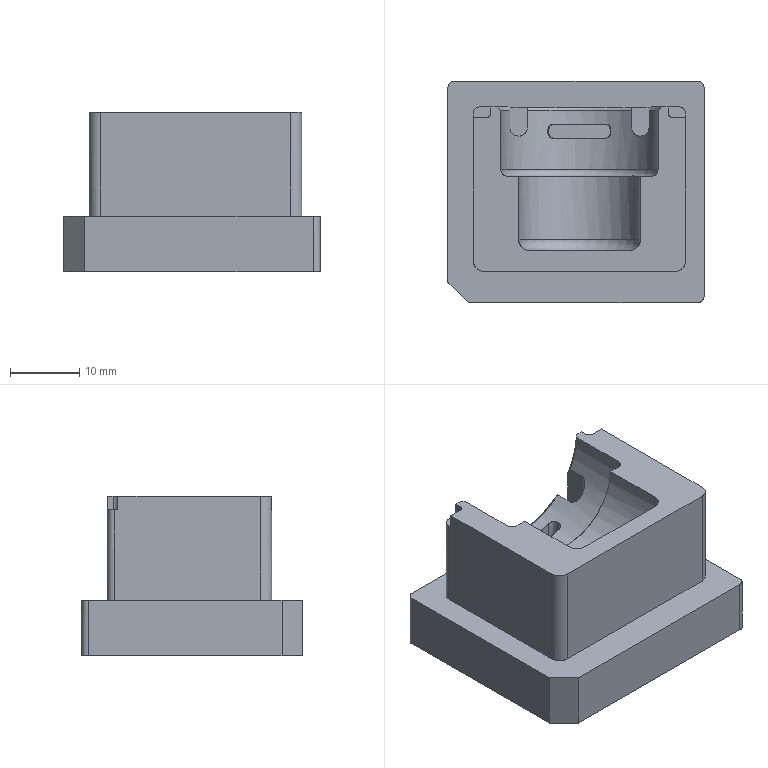NC program | PowerMill | posted with a generic post | part box 37 x 32 x 23 mm
Lines 5912 to 6889 of 253511:
N6009 M6
N6010 S18000 M03
N6011 G00 G90 X0.0 Y0.0
N6012 G43 Z9.8 H15
N6013
N6014 G05 P10000 R4
N6015 X1.851 Y-13.9296
N6016 Z0.8426
N6017 G01 Z-0.3574 F3000.0
N6018 X1.8596 Y-13.9124 F5000.0
N6019 G03 X1.7821 Y-13.6799 I-0.155 J0.0775
N6020 G01 X0.4221 Y-12.9999
N6021 X-13.0861
N6022 X-13.5083 Y-12.9833
N6023 X-13.9304 Y-12.9241
N6024 X-14.3525 Y-12.8
N6025 X-14.7747 Y-12.6037
N6026 X-15.1968 Y-12.3085
N6027 X-15.6189 Y-11.8974
N6028 X-15.9721 Y-11.3976
N6029 X-16.1651 Y-10.9755
N6030 X-16.2874 Y-10.5533
N6031 X-16.3436 Y-10.1312
N6032 X-16.3585 Y-9.7091
N6033 Y10.5533
N6034 X-16.3332 Y10.9755
N6035 X-16.1868 Y11.3976
N6036 X-16.0411 Y11.6235
N6037 X-15.8575 Y11.8197
N6038 X-15.6189 Y11.9937
N6039 X-15.1968 Y12.1621
N6040 X-14.7747 Y12.2007
N6041 X-13.9496
N6042 X-13.8965 Y12.2105
N6043 X-13.8503 Y12.2384
N6044 X-13.8336 Y12.2595
N6045 X-13.8169 Y12.2808
N6046 X-13.8007 Y12.3323
N6047 X-13.7597 Y12.664
N6048 X-13.5651 Y13.0861
N6049 X-13.5083 Y13.1658
N6050 X-13.1402 Y13.5083
N6051 X-12.664 Y13.7137
N6052 X-12.2419 Y13.7545
N6053 X-11.3976
N6054 X-10.9755 Y13.7073
N6055 X-10.5533 Y13.5265
N6056 X-10.1312 Y13.1593
N6057 X-9.7091 Y12.7315
N6058 X-9.4273 Y12.2419
N6059 X-9.3466 Y11.8197
N6060 X-9.3448 Y3.8549
N6061 G03 X-9.1949 Y3.7049 I0.15 J0.0
N6062 G01 X-8.4427 Y3.7045
N6063 X-8.0205 Y3.6777
N6064 X-7.5984 Y3.5401
N6065 X-7.3433 Y3.3771
N6066 X-7.1763 Y3.2216
N6067 X-6.98 Y2.9549
N6068 X-6.8151 Y2.5328
N6069 X-6.7788 Y2.1107
N6070 X-6.7766 Y-6.8379
N6071 G03 X-6.6267 Y-6.9878 I0.15 J0.0001
N6072 G01 X7.5984 Y-7.0024
N6073 X7.6758 Y-6.9844
N6074 X7.7408 Y-6.9386
N6075 X7.7658 Y-6.8942
N6076 X7.7745 Y-6.8439
N6077 X7.7746 Y2.1107
N6078 X7.8108 Y2.5328
N6079 X7.9758 Y2.9549
N6080 X8.3392 Y3.3771
N6081 X8.4427 Y3.4524
N6082 X8.8648 Y3.6473
N6083 X9.2869 Y3.7045
N6084 X10.1905
N6085 G03 X10.3405 Y3.8545 I0.0 J0.15
N6086 G01 X10.3425 Y11.8197
N6087 X10.4231 Y12.2419
N6088 X10.5533 Y12.5205
N6089 X10.65 Y12.664
N6090 X11.3976 Y13.418
N6091 X11.5206 Y13.5083
N6092 X11.8197 Y13.6569
N6093 X12.2419 Y13.7507
N6094 X13.5083 Y13.7416
N6095 X13.9304 Y13.6214
N6096 X14.1361 Y13.5083
N6097 X14.3525 Y13.3355
N6098 X14.561 Y13.0861
N6099 X14.7557 Y12.664
N6100 X14.7965 Y12.3326
N6101 G03 X14.9453 Y12.2009 I0.1489 J0.0183
N6102 G01 X15.4933 Y12.2025
N6103 X16.0411 Y12.189
N6104 X16.4632 Y12.0717
N6105 X16.8533 Y11.8197
N6106 X17.1827 Y11.3976
N6107 X17.3075 Y11.0731
N6108 X17.3544 Y10.5533
N6109 Y-9.7091
N6110 X17.3075 Y-10.4367
N6111 X17.161 Y-10.9755
N6112 X16.8853 Y-11.5381
N6113 X16.4632 Y-12.0749
N6114 X16.0411 Y-12.4308
N6115 X15.6461 Y-12.664
N6116 X15.1968 Y-12.8494
N6117 X14.7747 Y-12.9556
N6118 X14.3525 Y-12.9967
N6119 X13.9304 Y-12.9999
N6120 X0.4221
N6121 X1.851 Y-13.9296 Z-0.5048
N6122 X1.8596 Y-13.9124
N6123 G03 X1.7821 Y-13.6799 I-0.155 J0.0775
N6124 G01 X0.4221 Y-12.9999
N6125 X-13.0861
N6126 X-13.5083 Y-12.9833
N6127 X-13.9304 Y-12.9241
N6128 X-14.3525 Y-12.8
N6129 X-14.7747 Y-12.6037
N6130 X-15.1968 Y-12.3085
N6131 X-15.6189 Y-11.8974
N6132 X-15.9721 Y-11.3976
N6133 X-16.1651 Y-10.9755
N6134 X-16.2874 Y-10.5533
N6135 X-16.3436 Y-10.1312
N6136 X-16.3585 Y-9.7091
N6137 Y10.5533
N6138 X-16.3332 Y10.9755
N6139 X-16.1868 Y11.3976
N6140 X-16.0411 Y11.6235
N6141 X-15.8575 Y11.8197
N6142 X-15.6189 Y11.9937
N6143 X-15.1968 Y12.1621
N6144 X-14.7747 Y12.2008
N6145 X-13.9496
N6146 G03 X-13.8007 Y12.3323 I0.0 J0.15
N6147 G01 X-13.7597 Y12.664
N6148 X-13.5651 Y13.0861
N6149 X-13.5083 Y13.1658
N6150 X-13.1402 Y13.5083
N6151 X-12.664 Y13.7137
N6152 X-12.2419 Y13.7545
N6153 X-11.3976
N6154 X-10.9755 Y13.7097
N6155 X-10.5533 Y13.5324
N6156 X-10.1312 Y13.1691
N6157 X-9.7118 Y12.7342
N6158 X-9.7091 Y12.7315
N6159 X-9.709 Y12.7313
N6160 X-9.6441 Y12.664
N6161 X-9.4172 Y12.2419
N6162 X-9.3365 Y11.8197
N6163 X-9.3345 Y3.8547
N6164 G03 X-9.191 Y3.7049 I0.15 J0.0
N6165 G01 X-8.6479 Y3.7046
N6166 X-8.4427 Y3.7045
N6167 X-8.0205 Y3.6812
N6168 X-7.5984 Y3.5477
N6169 X-7.3307 Y3.3771
N6170 X-7.1763 Y3.2349
N6171 X-6.9673 Y2.9549
N6172 X-6.8025 Y2.5328
N6173 X-6.7661 Y2.1107
N6174 X-6.7657 Y-6.8448
N6175 X-6.7625 Y-6.8644
N6176 X-6.7197 Y-6.9464
N6177 X-6.6365 Y-6.9866
N6178 X-6.6267 Y-6.9879
N6179 X5.9184 Y-7.0008
N6180 X7.5912 Y-7.0009
N6181 X7.6062 Y-7.0001
N6182 X7.621 Y-6.9978
N6183 X7.6432 Y-6.9933
N6184 X7.7205 Y-6.9501
N6185 X7.759 Y-6.8703
N6186 X7.762 Y-6.8489
N6187 Y2.1107
N6188 X7.7979 Y2.5328
N6189 X7.9632 Y2.9549
N6190 X8.0205 Y3.0455
N6191 X8.3265 Y3.3771
N6192 X8.4427 Y3.4605
N6193 X8.8648 Y3.6507
N6194 X9.2869 Y3.7045
N6195 X10.1802
N6196 G03 X10.3302 Y3.8545 I0.0 J0.15
N6197 G01 X10.3324 Y11.8197
N6198 X10.4128 Y12.2419
N6199 X10.5533 Y12.5366
N6200 X10.6399 Y12.664
N6201 X11.3976 Y13.4257
N6202 X11.5107 Y13.5083
N6203 X11.8197 Y13.6635
N6204 X12.2419 Y13.7514
N6205 X13.5083 Y13.7416
N6206 X13.9304 Y13.6214
N6207 X14.1361 Y13.5083
N6208 X14.3525 Y13.3356
N6209 X14.561 Y13.0861
N6210 X14.7557 Y12.664
N6211 X14.7965 Y12.3326
N6212 G03 X14.9453 Y12.201 I0.1489 J0.0183
N6213 G01 X15.4933 Y12.2025
N6214 X16.0411 Y12.189
N6215 X16.4632 Y12.0717
N6216 X16.8533 Y11.8197
N6217 X17.1827 Y11.3976
N6218 X17.3075 Y11.0731
N6219 X17.3544 Y10.5533
N6220 Y-9.7091
N6221 X17.3075 Y-10.4367
N6222 X17.161 Y-10.9755
N6223 X16.8853 Y-11.5381
N6224 X16.4632 Y-12.0749
N6225 X16.0411 Y-12.4308
N6226 X15.6461 Y-12.664
N6227 X15.1968 Y-12.8494
N6228 X14.7747 Y-12.9556
N6229 X14.3525 Y-12.9967
N6230 X13.9304 Y-12.9999
N6231 X0.4221
N6232 X1.851 Y-13.9296 Z-0.6521
N6233 X1.8596 Y-13.9124
N6234 G03 X1.7821 Y-13.6799 I-0.155 J0.0775
N6235 G01 X0.4221 Y-12.9999
N6236 X-13.0861
N6237 X-13.5083 Y-12.9833
N6238 X-13.9304 Y-12.9241
N6239 X-14.3525 Y-12.8
N6240 X-14.7747 Y-12.6037
N6241 X-15.1968 Y-12.3085
N6242 X-15.6189 Y-11.8974
N6243 X-15.9721 Y-11.3976
N6244 X-16.1651 Y-10.9755
N6245 X-16.2874 Y-10.5533
N6246 X-16.3436 Y-10.1312
N6247 X-16.3585 Y-9.7091
N6248 Y10.5533
N6249 X-16.3332 Y10.9755
N6250 X-16.1868 Y11.3976
N6251 X-16.0411 Y11.6235
N6252 X-15.8575 Y11.8197
N6253 X-15.6189 Y11.9937
N6254 X-15.1968 Y12.1621
N6255 X-14.7747 Y12.2008
N6256 X-13.9496
N6257 G03 X-13.8007 Y12.3324 I0.0 J0.15
N6258 G01 X-13.7598 Y12.664
N6259 X-13.5651 Y13.0861
N6260 X-13.5083 Y13.1658
N6261 X-13.1402 Y13.5083
N6262 X-12.664 Y13.7137
N6263 X-12.2419 Y13.7545
N6264 X-11.3976
N6265 X-10.9755 Y13.712
N6266 X-10.5533 Y13.5384
N6267 X-10.1312 Y13.1788
N6268 X-9.634 Y12.664
N6269 X-9.4071 Y12.2419
N6270 X-9.3264 Y11.8197
N6271 X-9.3242 Y3.8524
N6272 X-9.312 Y3.7924
N6273 X-9.2746 Y3.7438
N6274 X-9.2285 Y3.7149
N6275 X-9.175 Y3.7048
N6276 X-8.6479 Y3.7045
N6277 X-8.3341 Y3.6997
N6278 X-8.0205 Y3.6847
N6279 X-7.5984 Y3.5539
N6280 X-7.318 Y3.3771
N6281 X-7.1763 Y3.2483
N6282 X-6.9547 Y2.9549
N6283 X-6.7898 Y2.5328
N6284 X-6.7541 Y2.248
N6285 X-6.7532 Y-6.8394
N6286 G03 X-6.6239 Y-6.9879 I0.15 J0.0
N6287 G01 X4.5985 Y-6.9995
N6288 X7.5871 Y-6.9993
N6289 X7.6098 Y-6.9975
N6290 X7.6319 Y-6.9923
N6291 G03 X7.7487 Y-6.848 I-0.0282 J0.1422
N6292 G01 X7.7494 Y2.1107
N6293 X7.785 Y2.5328
N6294 X7.9506 Y2.9549
N6295 X8.0205 Y3.0642
N6296 X8.3139 Y3.3771
N6297 X8.4427 Y3.4685
N6298 X8.8648 Y3.6541
N6299 X9.2869 Y3.7045
N6300 X10.1701
N6301 G03 X10.3201 Y3.8545 I0.0 J0.15
N6302 G01 X10.3223 Y11.8197
N6303 X10.4026 Y12.2419
N6304 X10.4816 Y12.3874
N6305 X10.5534 Y12.5366
N6306 X10.5949 Y12.5983
N6307 X10.6299 Y12.664
N6308 X10.9755 Y13.027
N6309 X11.2635 Y13.2908
N6310 X11.3976 Y13.4256
N6311 X11.4623 Y13.4729
N6312 X11.501 Y13.5083
N6313 X11.8197 Y13.6669
N6314 X12.2419 Y13.752
N6315 X13.5083 Y13.7416
N6316 X13.9304 Y13.6214
N6317 X14.1361 Y13.5083
N6318 X14.3525 Y13.3356
N6319 X14.561 Y13.0861
N6320 X14.7557 Y12.664
N6321 X14.7965 Y12.3326
N6322 G03 X14.9453 Y12.201 I0.1489 J0.0184
N6323 G01 X15.4933 Y12.2025
N6324 X16.0411 Y12.189
N6325 X16.4632 Y12.0717
N6326 X16.8533 Y11.8197
N6327 X17.1827 Y11.3976
N6328 X17.3075 Y11.0731
N6329 X17.3544 Y10.5533
N6330 Y-9.7091
N6331 X17.3075 Y-10.4367
N6332 X17.161 Y-10.9755
N6333 X16.8853 Y-11.5381
N6334 X16.4632 Y-12.0749
N6335 X16.0411 Y-12.4308
N6336 X15.6461 Y-12.664
N6337 X15.1968 Y-12.8494
N6338 X14.7747 Y-12.9556
N6339 X14.3525 Y-12.9967
N6340 X13.9304 Y-12.9999
N6341 X0.4221
N6342 X1.851 Y-13.9296 Z-0.7995
N6343 X1.8596 Y-13.9124
N6344 G03 X1.7821 Y-13.6799 I-0.155 J0.0775
N6345 G01 X0.4221 Y-12.9999
N6346 X-13.0861
N6347 X-13.5083 Y-12.9833
N6348 X-13.9304 Y-12.9241
N6349 X-14.3525 Y-12.8
N6350 X-14.7747 Y-12.6037
N6351 X-15.1968 Y-12.3085
N6352 X-15.6189 Y-11.8974
N6353 X-15.9721 Y-11.3976
N6354 X-16.1651 Y-10.9755
N6355 X-16.2874 Y-10.5533
N6356 X-16.3436 Y-10.1312
N6357 X-16.3585 Y-9.7091
N6358 Y10.5533
N6359 X-16.3332 Y10.9755
N6360 X-16.1869 Y11.3976
N6361 X-16.0411 Y11.6236
N6362 X-15.8575 Y11.8197
N6363 X-15.6189 Y11.9937
N6364 X-15.1968 Y12.1621
N6365 X-14.7747 Y12.2008
N6366 X-13.9496
N6367 G03 X-13.8007 Y12.3324 I0.0 J0.15
N6368 G01 X-13.7598 Y12.664
N6369 X-13.5651 Y13.0861
N6370 X-13.5083 Y13.1658
N6371 X-13.1403 Y13.5083
N6372 X-12.664 Y13.7137
N6373 X-12.2419 Y13.7545
N6374 X-11.3976
N6375 X-10.9755 Y13.7144
N6376 X-10.5533 Y13.5443
N6377 X-10.1312 Y13.1886
N6378 X-9.6239 Y12.664
N6379 X-9.3971 Y12.2419
N6380 X-9.3164 Y11.8197
N6381 X-9.3139 Y3.853
N6382 X-9.2863 Y3.766
N6383 X-9.2117 Y3.7134
N6384 X-9.1866 Y3.7048
N6385 X-8.6034
N6386 X-8.0205 Y3.6882
N6387 X-7.5984 Y3.5602
N6388 X-7.3054 Y3.3771
N6389 X-7.1763 Y3.2617
N6390 X-6.942 Y2.9549
N6391 X-6.7772 Y2.5328
N6392 X-6.7408 Y2.1107
N6393 X-6.741 Y-6.8382
N6394 G03 X-6.5986 Y-6.988 I0.15 J0.0
N6395 G01 X3.5218 Y-6.9984
N6396 X7.5848 Y-6.9977
N6397 G03 X7.7348 Y-6.8478 I0.0 J0.15
N6398 G01 X7.7367 Y2.1107
N6399 X7.7721 Y2.5328
N6400 X7.9379 Y2.9549
N6401 X8.0205 Y3.0825
N6402 X8.3013 Y3.3771
N6403 X8.4427 Y3.4766
N6404 X8.8648 Y3.6575
N6405 X9.2869 Y3.7045
N6406 X10.1597
N6407 G03 X10.3097 Y3.8545 I0.0 J0.15
N6408 G01 X10.3122 Y11.8197
N6409 X10.3924 Y12.2419
N6410 X10.6198 Y12.664
N6411 X10.8271 Y12.8711
N6412 X10.9431 Y12.9951
N6413 X11.0673 Y13.111
N6414 X11.3976 Y13.441
N6415 X11.4713 Y13.481
N6416 X11.501 Y13.5082
N6417 X11.7434 Y13.6289
N6418 X11.8197 Y13.6703
N6419 X12.2419 Y13.7526
N6420 X13.5083 Y13.7416
N6421 X13.9304 Y13.6214
N6422 X14.1362 Y13.5083
N6423 X14.3525 Y13.3356
N6424 X14.561 Y13.0861
N6425 X14.7557 Y12.664
N6426 X14.7965 Y12.3326
N6427 G03 X14.9453 Y12.201 I0.1489 J0.0184
N6428 G01 X15.4933 Y12.2025
N6429 X16.0411 Y12.189
N6430 X16.4632 Y12.0717
N6431 X16.8533 Y11.8197
N6432 X17.1827 Y11.3976
N6433 X17.3075 Y11.0731
N6434 X17.3544 Y10.5533
N6435 Y-9.7091
N6436 X17.3075 Y-10.4367
N6437 X17.161 Y-10.9755
N6438 X16.8853 Y-11.5381
N6439 X16.4632 Y-12.0749
N6440 X16.0411 Y-12.4308
N6441 X15.6461 Y-12.664
N6442 X15.1968 Y-12.8494
N6443 X14.7747 Y-12.9556
N6444 X14.3525 Y-12.9967
N6445 X13.9304 Y-12.9999
N6446 X0.4221
N6447 X1.851 Y-13.9296 Z-0.9469
N6448 X1.8596 Y-13.9124
N6449 G03 X1.7821 Y-13.6799 I-0.155 J0.0775
N6450 G01 X0.4221 Y-12.9999
N6451 X-13.0861
N6452 X-13.5083 Y-12.9833
N6453 X-13.9304 Y-12.9241
N6454 X-14.3525 Y-12.8
N6455 X-14.7747 Y-12.6037
N6456 X-15.1968 Y-12.3085
N6457 X-15.6189 Y-11.8974
N6458 X-15.9721 Y-11.3976
N6459 X-16.1651 Y-10.9755
N6460 X-16.2874 Y-10.5533
N6461 X-16.3436 Y-10.1312
N6462 X-16.3585 Y-9.7091
N6463 Y10.5533
N6464 X-16.3332 Y10.9755
N6465 X-16.1869 Y11.3976
N6466 X-16.0411 Y11.6236
N6467 X-15.8575 Y11.8197
N6468 X-15.6189 Y11.9937
N6469 X-15.1968 Y12.1621
N6470 X-14.7747 Y12.2008
N6471 X-13.9496
N6472 G03 X-13.8007 Y12.3324 I0.0 J0.15
N6473 G01 X-13.7598 Y12.664
N6474 X-13.5651 Y13.0861
N6475 X-13.5083 Y13.1658
N6476 X-13.1403 Y13.5083
N6477 X-12.664 Y13.7137
N6478 X-12.2419 Y13.7545
N6479 X-11.3976
N6480 X-10.9755 Y13.7168
N6481 X-10.5533 Y13.5502
N6482 X-10.1312 Y13.1983
N6483 X-9.6138 Y12.664
N6484 X-9.387 Y12.2419
N6485 X-9.3063 Y11.8197
N6486 X-9.3035 Y3.8533
N6487 G03 X-9.1735 Y3.7047 I0.15 J0.0001
N6488 G01 X-8.5969 Y3.7042
N6489 X-8.0205 Y3.6905
N6490 X-7.5984 Y3.5664
N6491 X-7.2927 Y3.3771
N6492 X-7.1763 Y3.275
N6493 X-6.9294 Y2.9549
N6494 X-6.7646 Y2.5328
N6495 X-6.7282 Y2.1107
N6496 X-6.7284 Y-6.8351
N6497 G03 X-6.5956 Y-6.9841 I0.15 J0.0
N6498 G01 X-6.5608 Y-6.9881
N6499 X3.5218 Y-6.9985
N6500 X6.9075 Y-6.9979
N6501 X7.5757 Y-6.9887
N6502 G03 X7.7237 Y-6.8387 I-0.002 J0.15
N6503 G01 X7.7241 Y2.1107
N6504 X7.7593 Y2.5328
N6505 X7.9253 Y2.9549
N6506 X8.0205 Y3.1001
N6507 X8.2886 Y3.3771
N6508 X8.4427 Y3.4847
N6509 X8.8648 Y3.6614
N6510 X9.2869 Y3.7045
N6511 X10.1496
N6512 G03 X10.2996 Y3.8545 I0.0 J0.15
N6513 G01 X10.3022 Y11.8197
N6514 X10.3821 Y12.2419
N6515 X10.6097 Y12.664
N6516 X11.3976 Y13.4486
N6517 X11.4733 Y13.489
N6518 X11.4877 Y13.4978
N6519 X11.501 Y13.5082
N6520 X11.6241 Y13.5694
N6521 X11.8197 Y13.6737
N6522 X12.2419 Y13.7532
N6523 X13.5083 Y13.7416
N6524 X13.9304 Y13.6215
N6525 X14.1362 Y13.5083
N6526 X14.3525 Y13.3356
N6527 X14.561 Y13.0861
N6528 X14.7557 Y12.664
N6529 X14.7965 Y12.3326
N6530 G03 X14.9453 Y12.201 I0.1489 J0.0184
N6531 G01 X15.4933 Y12.2025
N6532 X16.0411 Y12.1891
N6533 X16.4632 Y12.0717
N6534 X16.8533 Y11.8197
N6535 X17.1827 Y11.3976
N6536 X17.3075 Y11.0731
N6537 X17.3544 Y10.5533
N6538 Y-9.7091
N6539 X17.3075 Y-10.4367
N6540 X17.161 Y-10.9755
N6541 X16.8853 Y-11.5381
N6542 X16.4632 Y-12.075
N6543 X16.0411 Y-12.4308
N6544 X15.6461 Y-12.664
N6545 X15.1968 Y-12.8494
N6546 X14.7747 Y-12.9556
N6547 X14.3525 Y-12.9967
N6548 X13.9304 Y-12.9999
N6549 X0.4221
N6550 X1.851 Y-13.9296 Z-1.0943
N6551 X1.8596 Y-13.9124
N6552 G03 X1.7821 Y-13.6799 I-0.155 J0.0775
N6553 G01 X0.4221 Y-12.9999
N6554 X-13.0861
N6555 X-13.5083 Y-12.9833
N6556 X-13.9304 Y-12.9241
N6557 X-14.3525 Y-12.8
N6558 X-14.7747 Y-12.6037
N6559 X-15.1968 Y-12.3085
N6560 X-15.6189 Y-11.8974
N6561 X-15.9721 Y-11.3976
N6562 X-16.1651 Y-10.9755
N6563 X-16.2874 Y-10.5533
N6564 X-16.3436 Y-10.1312
N6565 X-16.3586 Y-9.7091
N6566 Y10.5533
N6567 X-16.3332 Y10.9755
N6568 X-16.1869 Y11.3976
N6569 X-16.0411 Y11.6236
N6570 X-15.8575 Y11.8197
N6571 X-15.6189 Y11.9937
N6572 X-15.1968 Y12.1621
N6573 X-14.7747 Y12.2008
N6574 X-13.9496
N6575 G03 X-13.8008 Y12.3324 I0.0 J0.15
N6576 G01 X-13.7598 Y12.664
N6577 X-13.5651 Y13.0861
N6578 X-13.5083 Y13.1658
N6579 X-13.1403 Y13.5083
N6580 X-12.664 Y13.7138
N6581 X-12.2419 Y13.7545
N6582 X-11.3976
N6583 X-10.9755 Y13.7191
N6584 X-10.5533 Y13.5571
N6585 X-10.1312 Y13.2081
N6586 X-9.6038 Y12.664
N6587 X-9.3769 Y12.2419
N6588 X-9.2962 Y11.8197
N6589 X-9.2932 Y3.8546
N6590 G03 X-9.1463 Y3.7047 I0.15 J0.0
N6591 G01 X-8.5834 Y3.7037
N6592 X-8.0205 Y3.6927
N6593 X-7.5984 Y3.5727
N6594 X-7.2799 Y3.3771
N6595 X-7.1763 Y3.2884
N6596 X-6.9147 Y2.9549
N6597 X-6.7503 Y2.5328
N6598 X-6.7156 Y2.1107
N6599 Y-6.7541
N6600 X-6.7143 Y-6.8221
N6601 X-6.7014 Y-6.8889
N6602 X-6.6551 Y-6.9505
N6603 X-6.5843 Y-6.9809
N6604 X-6.5352 Y-6.9882
N6605 X3.5218 Y-6.9985
N6606 X6.9075 Y-6.998
N6607 X7.5555 Y-6.9891
N6608 X7.6429 Y-6.9588
N6609 X7.6949 Y-6.8824
N6610 X7.7019 Y-6.8578
N6611 X7.711 Y-6.7541
N6612 X7.7114 Y2.1107
N6613 X7.7464 Y2.5328
N6614 X7.9111 Y2.9549
N6615 X8.0205 Y3.1177
N6616 X8.274 Y3.3771
N6617 X8.4427 Y3.4948
N6618 X8.8648 Y3.6662
N6619 X9.2869 Y3.7045
N6620 X10.1398
N6621 G03 X10.2898 Y3.8545 I0.0 J0.15
N6622 G01 X10.2921 Y11.8197
N6623 X10.3719 Y12.2419
N6624 X10.5996 Y12.664
N6625 X11.3976 Y13.4565
N6626 X11.8197 Y13.6777
N6627 X12.2419 Y13.7535
N6628 X13.5083 Y13.7417
N6629 X13.9304 Y13.6215
N6630 X14.1362 Y13.5083
N6631 X14.3525 Y13.3356
N6632 X14.561 Y13.0861
N6633 X14.7557 Y12.664
N6634 X14.7965 Y12.3326
N6635 G03 X14.9453 Y12.201 I0.1489 J0.0184
N6636 G01 X15.4933 Y12.2025
N6637 X16.0411 Y12.1891
N6638 X16.4632 Y12.0717
N6639 X16.8534 Y11.8197
N6640 X17.1827 Y11.3976
N6641 X17.3075 Y11.0731
N6642 X17.3544 Y10.5533
N6643 Y-9.7091
N6644 X17.3075 Y-10.4367
N6645 X17.161 Y-10.9755
N6646 X16.8853 Y-11.5381
N6647 X16.4632 Y-12.075
N6648 X16.0411 Y-12.4308
N6649 X15.6461 Y-12.664
N6650 X15.1968 Y-12.8494
N6651 X14.7747 Y-12.9556
N6652 X14.3525 Y-12.9967
N6653 X13.9304 Y-12.9999
N6654 X0.4221
N6655 X1.851 Y-13.9296 Z-1.2417
N6656 X1.8596 Y-13.9124
N6657 G03 X1.7821 Y-13.6799 I-0.155 J0.0775
N6658 G01 X0.4221 Y-12.9999
N6659 X-13.0861
N6660 X-13.5083 Y-12.9833
N6661 X-13.9304 Y-12.9241
N6662 X-14.3525 Y-12.8
N6663 X-14.7747 Y-12.6037
N6664 X-15.1968 Y-12.3085
N6665 X-15.6189 Y-11.8974
N6666 X-15.9721 Y-11.3976
N6667 X-16.1651 Y-10.9755
N6668 X-16.2874 Y-10.5533
N6669 X-16.3436 Y-10.1312
N6670 X-16.3586 Y-9.7091
N6671 Y10.5533
N6672 X-16.3332 Y10.9755
N6673 X-16.1869 Y11.3976
N6674 X-16.0411 Y11.6236
N6675 X-15.8575 Y11.8197
N6676 X-15.6189 Y11.9937
N6677 X-15.1968 Y12.1621
N6678 X-14.7747 Y12.2008
N6679 X-13.9496
N6680 G03 X-13.8008 Y12.3324 I0.0 J0.15
N6681 G01 X-13.7598 Y12.664
N6682 X-13.5651 Y13.0861
N6683 X-13.5083 Y13.1658
N6684 X-13.1403 Y13.5083
N6685 X-12.664 Y13.7138
N6686 X-12.2419 Y13.7545
N6687 X-11.3976
N6688 X-10.9755 Y13.7225
N6689 X-10.5533 Y13.5641
N6690 X-10.1312 Y13.2195
N6691 X-9.5931 Y12.664
N6692 X-9.3646 Y12.2419
N6693 X-9.2869 Y11.8361
N6694 X-9.2825 Y11.3976
N6695 X-9.2829 Y3.8535
N6696 G03 X-9.1742 Y3.7118 I0.1433 J-0.0026
N6697 G01 X-9.1519 Y3.7064
N6698 X-9.1289 Y3.7046
N6699 X-8.5747 Y3.7035
N6700 X-8.0205 Y3.695
N6701 X-7.5984 Y3.5822
N6702 X-7.3218 Y3.4027
N6703 X-7.2799 Y3.377
N6704 X-7.2729 Y3.371
N6705 X-7.1763 Y3.3083
N6706 X-6.8929 Y2.9549
N6707 X-6.7541 Y2.6292
N6708 X-6.6947 Y2.1107
N6709 X-6.6981 Y1.6885
N6710 Y-6.7541
N6711 X-6.6922 Y-6.8527
N6712 X-6.6829 Y-6.8834
N6713 X-6.6744 Y-6.9015
N6714 X-6.629 Y-6.9568
N6715 X-6.5629 Y-6.9841
N6716 X-6.5352 Y-6.9882
N6717 X3.5218 Y-6.9986
N6718 X6.9075 Y-6.998
N6719 X7.5347 Y-6.9894
N6720 X7.6218 Y-6.9593
N6721 X7.6739 Y-6.8833
N6722 X7.6801 Y-6.8615
N6723 X7.694 Y-6.7541
N6724 Y1.2664
N6725 X7.6904 Y2.1107
N6726 X7.7242 Y2.5328
N6727 X7.8889 Y2.9549
N6728 X8.0205 Y3.1461
N6729 X8.2529 Y3.3771
N6730 X8.4427 Y3.5069
N6731 X8.8648 Y3.6709
N6732 X9.2869 Y3.7045
N6733 X10.1293
N6734 G03 X10.2793 Y3.8545 I0.0 J0.15
N6735 G01 X10.279 Y11.8197
N6736 X10.3614 Y12.2419
N6737 X10.5862 Y12.664
N6738 X11.3976 Y13.4672
N6739 X11.8197 Y13.6834
N6740 X12.2419 Y13.754
N6741 X13.5083 Y13.7417
N6742 X13.9304 Y13.6215
N6743 X14.1362 Y13.5083
N6744 X14.3525 Y13.3356
N6745 X14.561 Y13.0861
N6746 X14.7558 Y12.664
N6747 X14.7965 Y12.3326
N6748 G03 X14.9453 Y12.201 I0.1489 J0.0184
N6749 G01 X15.4933 Y12.2026
N6750 X16.0411 Y12.1891
N6751 X16.4632 Y12.0717
N6752 X16.8534 Y11.8197
N6753 X17.1828 Y11.3976
N6754 X17.3075 Y11.0731
N6755 X17.3544 Y10.5533
N6756 Y-9.7091
N6757 X17.3075 Y-10.4367
N6758 X17.161 Y-10.9755
N6759 X16.8853 Y-11.5381
N6760 X16.4632 Y-12.075
N6761 X16.0411 Y-12.4308
N6762 X15.6461 Y-12.664
N6763 X15.1968 Y-12.8494
N6764 X14.7747 Y-12.9556
N6765 X14.3525 Y-12.9967
N6766 X13.9304 Y-12.9999
N6767 X0.4221
N6768 X1.851 Y-13.9296 Z-1.3891
N6769 X1.8596 Y-13.9124
N6770 G03 X1.7821 Y-13.6799 I-0.155 J0.0775
N6771 G01 X0.4221 Y-12.9999
N6772 X-13.0861
N6773 X-13.5083 Y-12.9833
N6774 X-13.9304 Y-12.9241
N6775 X-14.3525 Y-12.8
N6776 X-14.7747 Y-12.6037
N6777 X-15.1968 Y-12.3085
N6778 X-15.6189 Y-11.8974
N6779 X-15.9721 Y-11.3976
N6780 X-16.1651 Y-10.9755
N6781 X-16.2874 Y-10.5533
N6782 X-16.3436 Y-10.1312
N6783 X-16.3586 Y-9.7091
N6784 Y10.5533
N6785 X-16.3332 Y10.9755
N6786 X-16.1869 Y11.3976
N6787 X-16.0411 Y11.6236
N6788 X-15.8575 Y11.8197
N6789 X-15.6189 Y11.9937
N6790 X-15.1968 Y12.1622
N6791 X-14.7747 Y12.2008
N6792 X-13.9496
N6793 G03 X-13.8008 Y12.3324 I0.0 J0.15
N6794 G01 X-13.7598 Y12.664
N6795 X-13.5651 Y13.0861
N6796 X-13.5083 Y13.1658
N6797 X-13.1403 Y13.5083
N6798 X-12.664 Y13.7138
N6799 X-12.2419 Y13.7545
N6800 X-11.3976
N6801 X-10.9755 Y13.7259
N6802 X-10.5533 Y13.5745
N6803 X-10.4422 Y13.5083
N6804 X-10.1312 Y13.2384
N6805 X-9.57 Y12.664
N6806 X-9.3432 Y12.2419
N6807 X-9.2869 Y12.0288
N6808 X-9.2625 Y11.8197
N6809 X-9.2624 Y3.854
N6810 G03 X-9.1257 Y3.7045 I0.15 J0.0
N6811 G01 X-8.7396 Y3.7057
N6812 X-8.3534 Y3.6993
N6813 X-8.0205 Y3.6972
N6814 X-7.5984 Y3.5929
N6815 X-7.2328 Y3.3771
N6816 X-6.8689 Y2.9549
N6817 X-6.7541 Y2.704
N6818 X-6.7036 Y2.5328
N6819 X-6.6683 Y2.1107
N6820 Y-6.8412
N6821 X-6.6646 Y-6.8644
N6822 G03 X-6.5195 Y-6.9883 I0.1452 J0.0231
N6823 G01 X3.5218 Y-6.9986
N6824 X6.9075 Y-6.9981
N6825 X7.5145 Y-6.9897
N6826 X7.5876 Y-6.9691
N6827 X7.6406 Y-6.9148
N6828 X7.6575 Y-6.8804
N6829 X7.6618 Y-6.8423
N6830 X7.6641 Y2.1107
N6831 X7.7005 Y2.5328
N6832 X7.865 Y2.9549
N6833 X8.0205 Y3.1755
N6834 X8.2283 Y3.3771
N6835 X8.4427 Y3.5194
N6836 X8.8648 Y3.6757
N6837 X9.2869 Y3.7045
N6838 X10.1067
N6839 G03 X10.2567 Y3.8545 I0.0 J0.15
N6840 G01 X10.2572 Y11.8197
N6841 X10.3378 Y12.2419
N6842 X10.5647 Y12.664
N6843 X10.9718 Y13.0861
N6844 X11.3976 Y13.4809
N6845 X11.8197 Y13.6891
N6846 X12.2419 Y13.7544
N6847 X13.5083 Y13.7417
N6848 X13.9304 Y13.6215
N6849 X14.1362 Y13.5083
N6850 X14.3525 Y13.3356
N6851 X14.561 Y13.0861
N6852 X14.7558 Y12.664
N6853 X14.7965 Y12.3327
N6854 G03 X14.9453 Y12.201 I0.1489 J0.0183
N6855 G01 X15.4933 Y12.2026
N6856 X16.0411 Y12.1891
N6857 X16.4632 Y12.0717
N6858 X16.8534 Y11.8197
N6859 X17.1828 Y11.3976
N6860 X17.3075 Y11.0731
N6861 X17.3544 Y10.5533
N6862 Y-9.7091
N6863 X17.3075 Y-10.4367
N6864 X17.161 Y-10.9755
N6865 X16.8853 Y-11.5381
N6866 X16.4632 Y-12.075
N6867 X16.0411 Y-12.4308
N6868 X15.6461 Y-12.664
N6869 X15.1968 Y-12.8494
N6870 X14.7747 Y-12.9556
N6871 X14.3525 Y-12.9967
N6872 X13.9304 Y-12.9999
N6873 X0.4221
N6874 X1.851 Y-13.9296 Z-1.5365
N6875 X1.8596 Y-13.9124
N6876 G03 X1.7821 Y-13.6799 I-0.155 J0.0775
N6877 G01 X0.4221 Y-12.9999
N6878 X-13.0861
N6879 X-13.5083 Y-12.9833
N6880 X-13.9304 Y-12.9241
N6881 X-14.3525 Y-12.8
N6882 X-14.7747 Y-12.6037
N6883 X-15.1968 Y-12.3085
N6884 X-15.6189 Y-11.8974
N6885 X-15.9721 Y-11.3976
N6886 X-16.1651 Y-10.9755
N6887 X-16.2874 Y-10.5533
N6888 X-16.3436 Y-10.1312
N6889 X-16.3586 Y-9.7091
N6890 Y10.5533
N6891 X-16.3332 Y10.9755
N6892 X-16.1869 Y11.3976
N6893 X-16.0411 Y11.6236
N6894 X-15.8575 Y11.8197
N6895 X-15.6189 Y11.9937
N6896 X-15.1968 Y12.1622
N6897 X-14.7747 Y12.2008
N6898 X-13.9496
N6899 G03 X-13.8008 Y12.3324 I0.0 J0.15
N6900 G01 X-13.7598 Y12.664
N6901 X-13.5651 Y13.0861
N6902 X-13.5083 Y13.1658
N6903 X-13.1403 Y13.5083
N6904 X-12.664 Y13.7138
N6905 X-12.2419 Y13.7545
N6906 X-11.3976
N6907 X-10.9755 Y13.7294
N6908 X-10.5533 Y13.5855
N6909 X-10.4217 Y13.5083
N6910 X-10.1312 Y13.2616
N6911 X-9.5462 Y12.664
N6912 X-9.3193 Y12.2419
N6913 X-9.2386 Y11.8197
N6914 X-9.2378 Y3.8547
N6915 G03 X-9.0878 Y3.7047 I0.15 J0.0
N6916 G01 X-8.4427 Y3.7045
N6917 X-8.0205 Y3.6995
N6918 X-7.5984 Y3.6035
N6919 X-7.2029 Y3.3771
N6920 X-6.8396 Y2.9549
N6921 X-6.7541 Y2.7813
N6922 X-6.674 Y2.5328
N6923 X-6.6384 Y2.1107
N6924 X-6.6386 Y-6.8406
N6925 G03 X-6.5146 Y-6.9884 I0.15 J0.0
N6926 G01 X3.5218 Y-6.9987
N6927 X6.9075 Y-6.9981
N6928 X7.4864 Y-6.9901
N6929 G03 X7.6292 Y-6.8681 I-0.002 J0.1469
N6930 G01 X7.6336 Y-6.843
N6931 X7.6343 Y2.1107
N6932 X7.6707 Y2.5328
N6933 X7.8353 Y2.9549
N6934 X8.0205 Y3.2085
N6935 X8.1988 Y3.3771
N6936 X8.4427 Y3.5347
N6937 X8.8648 Y3.6804
N6938 X9.2869 Y3.7045
N6939 X10.0831
N6940 G03 X10.2331 Y3.8545 I0.0 J0.15
N6941 G01 X10.2335 Y11.8197
N6942 X10.3142 Y12.2419
N6943 X10.5411 Y12.664
N6944 X10.9486 Y13.0861
N6945 X11.3976 Y13.4956
N6946 X11.8197 Y13.6949
N6947 X12.2419 Y13.7545
N6948 X13.5083 Y13.7417
N6949 X13.9304 Y13.6215
N6950 X14.1362 Y13.5083
N6951 X14.3525 Y13.3356
N6952 X14.561 Y13.0861
N6953 X14.7558 Y12.664
N6954 X14.7965 Y12.3327
N6955 G03 X14.9454 Y12.201 I0.1489 J0.0183
N6956 G01 X15.4933 Y12.2026
N6957 X16.0411 Y12.1891
N6958 X16.4632 Y12.0717
N6959 X16.8534 Y11.8197
N6960 X17.1828 Y11.3976
N6961 X17.3075 Y11.0731
N6962 X17.3544 Y10.5533
N6963 Y-9.7091
N6964 X17.3075 Y-10.4367
N6965 X17.161 Y-10.9755
N6966 X16.8853 Y-11.5381
N6967 X16.4632 Y-12.075
N6968 X16.0411 Y-12.4308
N6969 X15.6461 Y-12.664
N6970 X15.1968 Y-12.8494
N6971 X14.7747 Y-12.9556
N6972 X14.3525 Y-12.9967
N6973 X13.9304 Y-12.9999
N6974 X0.4221
N6975 X1.851 Y-13.9296 Z-1.6838
N6976 X1.8596 Y-13.9124
N6977 G03 X1.7821 Y-13.6799 I-0.155 J0.0775
N6978 G01 X0.4221 Y-12.9999
N6979 X-13.0861
N6980 X-13.5083 Y-12.9833
N6981 X-13.9304 Y-12.9241
N6982 X-14.3525 Y-12.8
N6983 X-14.7747 Y-12.6037
N6984 X-15.1968 Y-12.3085
N6985 X-15.6189 Y-11.8974
N6986 X-15.9721 Y-11.3976